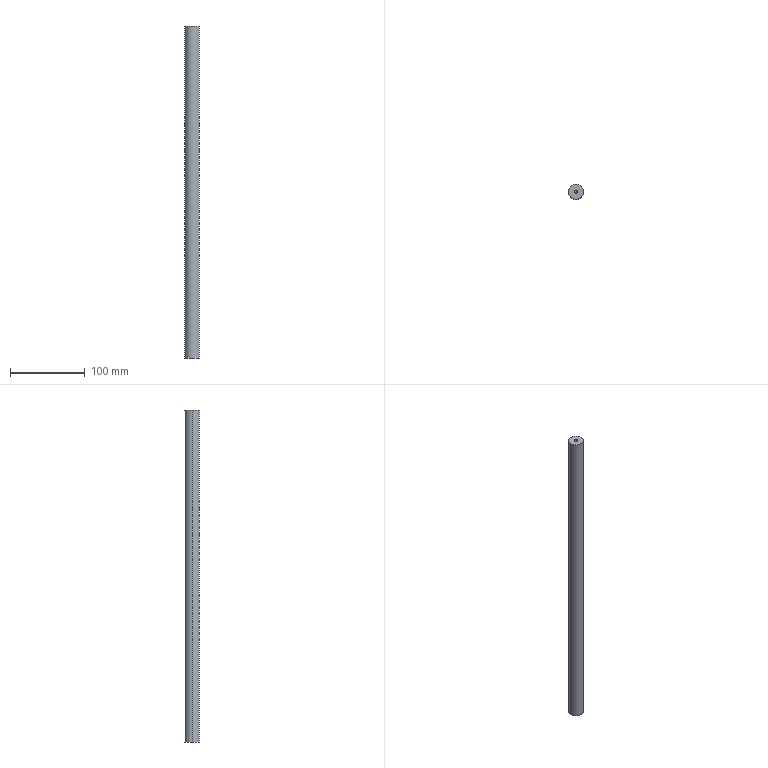Part | SolidWorks | features HoleWzd 2, Extrusion 1 | 1 solid | 12 faces | box 20 x 20 x 445 mm | volume 139374 mm3 | cylinder 6 | cone 4 | plane 2 | commonest cylinder face diameters 4.2 x4 20 x2
STEP:
#1=CARTESIAN_POINT('',(2.1,0.,15.));
#2=VERTEX_POINT('',#1);
#3=CARTESIAN_POINT('',(-2.1,0.,15.));
#4=VERTEX_POINT('',#3);
#5=CARTESIAN_POINT('',(0.,0.,15.));
#6=DIRECTION('',(0.,0.,-1.));
#7=DIRECTION('',(-1.,0.,0.));
#8=AXIS2_PLACEMENT_3D('',#5,#6,#7);
#9=CIRCLE('',#8,2.1);
#10=EDGE_CURVE('',#2,#4,#9,.T.);
#11=ORIENTED_EDGE('',*,*,#10,.F.);
#12=CARTESIAN_POINT('',(2.1,0.,0.));
#13=VERTEX_POINT('',#12);
#14=CARTESIAN_POINT('',(2.1,0.,0.));
#15=DIRECTION('',(0.,0.,-1.));
#16=VECTOR('',#15,1000.);
#17=LINE('',#14,#16);
#18=EDGE_CURVE('',#2,#13,#17,.T.);
#19=ORIENTED_EDGE('',*,*,#18,.T.);
#20=CARTESIAN_POINT('',(-2.1,0.,0.));
#21=VERTEX_POINT('',#20);
#22=CARTESIAN_POINT('',(0.,0.,0.));
#23=DIRECTION('',(0.,0.,-1.));
#24=DIRECTION('',(-1.,0.,0.));
#25=AXIS2_PLACEMENT_3D('',#22,#23,#24);
#26=CIRCLE('',#25,2.1);
#27=EDGE_CURVE('',#13,#21,#26,.T.);
#28=ORIENTED_EDGE('',*,*,#27,.T.);
#29=CARTESIAN_POINT('',(-2.1,0.,0.));
#30=DIRECTION('',(0.,0.,-1.));
#31=VECTOR('',#30,1000.);
#32=LINE('',#29,#31);
#33=EDGE_CURVE('',#4,#21,#32,.T.);
#34=ORIENTED_EDGE('',*,*,#33,.F.);
#35=EDGE_LOOP('',(#11,#19,#28,#34));
#36=FACE_OUTER_BOUND('',#35,.T.);
#37=CARTESIAN_POINT('',(0.,0.,0.));
#38=DIRECTION('',(0.,0.,-1.));
#39=DIRECTION('',(-1.,0.,0.));
#40=AXIS2_PLACEMENT_3D('',#37,#38,#39);
#41=CYLINDRICAL_SURFACE('',#40,2.1);
#42=ADVANCED_FACE('',(#36),#41,.F.);
#43=CARTESIAN_POINT('',(0.,0.,16.262));
#44=VERTEX_POINT('',#43);
#45=CARTESIAN_POINT('',(-2.1,0.,15.));
#46=DIRECTION('',(-0.8572,0.,-0.515));
#47=VECTOR('',#46,1000.);
#48=LINE('',#45,#47);
#49=EDGE_CURVE('',#44,#4,#48,.T.);
#50=ORIENTED_EDGE('',*,*,#49,.F.);
#51=CARTESIAN_POINT('',(2.1,0.,15.));
#52=DIRECTION('',(0.8572,0.,-0.515));
#53=VECTOR('',#52,1000.);
#54=LINE('',#51,#53);
#55=EDGE_CURVE('',#44,#2,#54,.T.);
#56=ORIENTED_EDGE('',*,*,#55,.T.);
#57=ORIENTED_EDGE('',*,*,#10,.T.);
#58=EDGE_LOOP('',(#50,#56,#57));
#59=FACE_OUTER_BOUND('',#58,.T.);
#60=CARTESIAN_POINT('',(0.,0.,15.));
#61=DIRECTION('',(0.,0.,-1.));
#62=DIRECTION('',(-1.,0.,0.));
#63=AXIS2_PLACEMENT_3D('',#60,#61,#62);
#64=CONICAL_SURFACE('',#63,2.1,1.03);
#65=ADVANCED_FACE('',(#59),#64,.F.);
#66=CARTESIAN_POINT('',(-2.1,0.,430.));
#67=VERTEX_POINT('',#66);
#68=CARTESIAN_POINT('',(2.1,0.,430.));
#69=VERTEX_POINT('',#68);
#70=CARTESIAN_POINT('',(0.,0.,430.));
#71=DIRECTION('',(0.,0.,1.));
#72=DIRECTION('',(1.,0.,0.));
#73=AXIS2_PLACEMENT_3D('',#70,#71,#72);
#74=CIRCLE('',#73,2.1);
#75=EDGE_CURVE('',#67,#69,#74,.T.);
#76=ORIENTED_EDGE('',*,*,#75,.F.);
#77=CARTESIAN_POINT('',(-2.1,0.,445.));
#78=VERTEX_POINT('',#77);
#79=CARTESIAN_POINT('',(-2.1,0.,445.));
#80=DIRECTION('',(0.,0.,1.));
#81=VECTOR('',#80,1000.);
#82=LINE('',#79,#81);
#83=EDGE_CURVE('',#67,#78,#82,.T.);
#84=ORIENTED_EDGE('',*,*,#83,.T.);
#85=CARTESIAN_POINT('',(2.1,0.,445.));
#86=VERTEX_POINT('',#85);
#87=CARTESIAN_POINT('',(0.,0.,445.));
#88=DIRECTION('',(0.,0.,1.));
#89=DIRECTION('',(1.,0.,0.));
#90=AXIS2_PLACEMENT_3D('',#87,#88,#89);
#91=CIRCLE('',#90,2.1);
#92=EDGE_CURVE('',#78,#86,#91,.T.);
#93=ORIENTED_EDGE('',*,*,#92,.T.);
#94=CARTESIAN_POINT('',(2.1,0.,445.));
#95=DIRECTION('',(0.,0.,1.));
#96=VECTOR('',#95,1000.);
#97=LINE('',#94,#96);
#98=EDGE_CURVE('',#69,#86,#97,.T.);
#99=ORIENTED_EDGE('',*,*,#98,.F.);
#100=EDGE_LOOP('',(#76,#84,#93,#99));
#101=FACE_OUTER_BOUND('',#100,.T.);
#102=CARTESIAN_POINT('',(0.,0.,445.));
#103=DIRECTION('',(0.,0.,1.));
#104=DIRECTION('',(1.,0.,0.));
#105=AXIS2_PLACEMENT_3D('',#102,#103,#104);
#106=CYLINDRICAL_SURFACE('',#105,2.1);
#107=ADVANCED_FACE('',(#101),#106,.F.);
#108=CARTESIAN_POINT('',(0.,0.,428.738));
#109=VERTEX_POINT('',#108);
#110=CARTESIAN_POINT('',(2.1,0.,430.));
#111=DIRECTION('',(0.8572,0.,0.515));
#112=VECTOR('',#111,1000.);
#113=LINE('',#110,#112);
#114=EDGE_CURVE('',#109,#69,#113,.T.);
#115=ORIENTED_EDGE('',*,*,#114,.F.);
#116=CARTESIAN_POINT('',(-2.1,0.,430.));
#117=DIRECTION('',(-0.8572,0.,0.515));
#118=VECTOR('',#117,1000.);
#119=LINE('',#116,#118);
#120=EDGE_CURVE('',#109,#67,#119,.T.);
#121=ORIENTED_EDGE('',*,*,#120,.T.);
#122=ORIENTED_EDGE('',*,*,#75,.T.);
#123=EDGE_LOOP('',(#115,#121,#122));
#124=FACE_OUTER_BOUND('',#123,.T.);
#125=CARTESIAN_POINT('',(0.,0.,430.));
#126=DIRECTION('',(0.,0.,1.));
#127=DIRECTION('',(1.,0.,0.));
#128=AXIS2_PLACEMENT_3D('',#125,#126,#127);
#129=CONICAL_SURFACE('',#128,2.1,1.03);
#130=ADVANCED_FACE('',(#124),#129,.F.);
#131=CARTESIAN_POINT('',(10.,0.,445.));
#132=VERTEX_POINT('',#131);
#133=CARTESIAN_POINT('',(-10.,0.,445.));
#134=VERTEX_POINT('',#133);
#135=CARTESIAN_POINT('',(0.,0.,445.));
#136=DIRECTION('',(0.,0.,1.));
#137=DIRECTION('',(1.,0.,0.));
#138=AXIS2_PLACEMENT_3D('',#135,#136,#137);
#139=CIRCLE('',#138,10.);
#140=EDGE_CURVE('',#132,#134,#139,.T.);
#141=ORIENTED_EDGE('',*,*,#140,.F.);
#142=CARTESIAN_POINT('',(10.,0.,0.));
#143=VERTEX_POINT('',#142);
#144=CARTESIAN_POINT('',(10.,0.,445.));
#145=DIRECTION('',(0.,0.,-1.));
#146=VECTOR('',#145,1000.);
#147=LINE('',#144,#146);
#148=EDGE_CURVE('',#132,#143,#147,.T.);
#149=ORIENTED_EDGE('',*,*,#148,.T.);
#150=CARTESIAN_POINT('',(-10.,0.,0.));
#151=VERTEX_POINT('',#150);
#152=CARTESIAN_POINT('',(0.,0.,0.));
#153=DIRECTION('',(0.,0.,1.));
#154=DIRECTION('',(1.,0.,0.));
#155=AXIS2_PLACEMENT_3D('',#152,#153,#154);
#156=CIRCLE('',#155,10.);
#157=EDGE_CURVE('',#143,#151,#156,.T.);
#158=ORIENTED_EDGE('',*,*,#157,.T.);
#159=CARTESIAN_POINT('',(-10.,0.,445.));
#160=DIRECTION('',(0.,0.,-1.));
#161=VECTOR('',#160,1000.);
#162=LINE('',#159,#161);
#163=EDGE_CURVE('',#134,#151,#162,.T.);
#164=ORIENTED_EDGE('',*,*,#163,.F.);
#165=EDGE_LOOP('',(#141,#149,#158,#164));
#166=FACE_OUTER_BOUND('',#165,.T.);
#167=CARTESIAN_POINT('',(0.,0.,445.));
#168=DIRECTION('',(0.,0.,-1.));
#169=DIRECTION('',(-1.,0.,0.));
#170=AXIS2_PLACEMENT_3D('',#167,#168,#169);
#171=CYLINDRICAL_SURFACE('',#170,10.);
#172=ADVANCED_FACE('',(#166),#171,.T.);
#173=ORIENTED_EDGE('',*,*,#148,.F.);
#174=CARTESIAN_POINT('',(0.,0.,445.));
#175=DIRECTION('',(0.,0.,1.));
#176=DIRECTION('',(1.,0.,0.));
#177=AXIS2_PLACEMENT_3D('',#174,#175,#176);
#178=CIRCLE('',#177,10.);
#179=EDGE_CURVE('',#134,#132,#178,.T.);
#180=ORIENTED_EDGE('',*,*,#179,.F.);
#181=ORIENTED_EDGE('',*,*,#163,.T.);
#182=CARTESIAN_POINT('',(0.,0.,0.));
#183=DIRECTION('',(0.,0.,1.));
#184=DIRECTION('',(1.,0.,0.));
#185=AXIS2_PLACEMENT_3D('',#182,#183,#184);
#186=CIRCLE('',#185,10.);
#187=EDGE_CURVE('',#151,#143,#186,.T.);
#188=ORIENTED_EDGE('',*,*,#187,.T.);
#189=EDGE_LOOP('',(#173,#180,#181,#188));
#190=FACE_OUTER_BOUND('',#189,.T.);
#191=CARTESIAN_POINT('',(0.,0.,445.));
#192=DIRECTION('',(0.,0.,-1.));
#193=DIRECTION('',(-1.,0.,0.));
#194=AXIS2_PLACEMENT_3D('',#191,#192,#193);
#195=CYLINDRICAL_SURFACE('',#194,10.);
#196=ADVANCED_FACE('',(#190),#195,.T.);
#197=CARTESIAN_POINT('',(0.,0.,445.));
#198=DIRECTION('',(0.,0.,1.));
#199=DIRECTION('',(1.,0.,0.));
#200=AXIS2_PLACEMENT_3D('',#197,#198,#199);
#201=CIRCLE('',#200,2.1);
#202=EDGE_CURVE('',#86,#78,#201,.T.);
#203=ORIENTED_EDGE('',*,*,#202,.F.);
#204=ORIENTED_EDGE('',*,*,#92,.F.);
#205=EDGE_LOOP('',(#203,#204));
#206=FACE_BOUND('',#205,.T.);
#207=ORIENTED_EDGE('',*,*,#179,.T.);
#208=ORIENTED_EDGE('',*,*,#140,.T.);
#209=EDGE_LOOP('',(#207,#208));
#210=FACE_OUTER_BOUND('',#209,.T.);
#211=CARTESIAN_POINT('',(0.,0.,445.));
#212=DIRECTION('',(0.,0.,1.));
#213=DIRECTION('',(1.,0.,0.));
#214=AXIS2_PLACEMENT_3D('',#211,#212,#213);
#215=PLANE('',#214);
#216=ADVANCED_FACE('',(#206,#210),#215,.T.);
#217=CARTESIAN_POINT('',(0.,0.,0.));
#218=DIRECTION('',(0.,0.,-1.));
#219=DIRECTION('',(-1.,0.,0.));
#220=AXIS2_PLACEMENT_3D('',#217,#218,#219);
#221=CIRCLE('',#220,2.1);
#222=EDGE_CURVE('',#21,#13,#221,.T.);
#223=ORIENTED_EDGE('',*,*,#222,.F.);
#224=ORIENTED_EDGE('',*,*,#27,.F.);
#225=EDGE_LOOP('',(#223,#224));
#226=FACE_BOUND('',#225,.T.);
#227=ORIENTED_EDGE('',*,*,#187,.F.);
#228=ORIENTED_EDGE('',*,*,#157,.F.);
#229=EDGE_LOOP('',(#227,#228));
#230=FACE_OUTER_BOUND('',#229,.T.);
#231=CARTESIAN_POINT('',(0.,0.,0.));
#232=DIRECTION('',(0.,0.,1.));
#233=DIRECTION('',(1.,0.,0.));
#234=AXIS2_PLACEMENT_3D('',#231,#232,#233);
#235=PLANE('',#234);
#236=ADVANCED_FACE('',(#226,#230),#235,.F.);
#237=ORIENTED_EDGE('',*,*,#120,.F.);
#238=ORIENTED_EDGE('',*,*,#114,.T.);
#239=CARTESIAN_POINT('',(0.,0.,430.));
#240=DIRECTION('',(0.,0.,1.));
#241=DIRECTION('',(1.,0.,0.));
#242=AXIS2_PLACEMENT_3D('',#239,#240,#241);
#243=CIRCLE('',#242,2.1);
#244=EDGE_CURVE('',#69,#67,#243,.T.);
#245=ORIENTED_EDGE('',*,*,#244,.T.);
#246=EDGE_LOOP('',(#237,#238,#245));
#247=FACE_OUTER_BOUND('',#246,.T.);
#248=CARTESIAN_POINT('',(0.,0.,430.));
#249=DIRECTION('',(0.,0.,1.));
#250=DIRECTION('',(1.,0.,0.));
#251=AXIS2_PLACEMENT_3D('',#248,#249,#250);
#252=CONICAL_SURFACE('',#251,2.1,1.03);
#253=ADVANCED_FACE('',(#247),#252,.F.);
#254=ORIENTED_EDGE('',*,*,#83,.F.);
#255=ORIENTED_EDGE('',*,*,#244,.F.);
#256=ORIENTED_EDGE('',*,*,#98,.T.);
#257=ORIENTED_EDGE('',*,*,#202,.T.);
#258=EDGE_LOOP('',(#254,#255,#256,#257));
#259=FACE_OUTER_BOUND('',#258,.T.);
#260=CARTESIAN_POINT('',(0.,0.,445.));
#261=DIRECTION('',(0.,0.,1.));
#262=DIRECTION('',(1.,0.,0.));
#263=AXIS2_PLACEMENT_3D('',#260,#261,#262);
#264=CYLINDRICAL_SURFACE('',#263,2.1);
#265=ADVANCED_FACE('',(#259),#264,.F.);
#266=ORIENTED_EDGE('',*,*,#55,.F.);
#267=ORIENTED_EDGE('',*,*,#49,.T.);
#268=CARTESIAN_POINT('',(0.,0.,15.));
#269=DIRECTION('',(0.,0.,-1.));
#270=DIRECTION('',(-1.,0.,0.));
#271=AXIS2_PLACEMENT_3D('',#268,#269,#270);
#272=CIRCLE('',#271,2.1);
#273=EDGE_CURVE('',#4,#2,#272,.T.);
#274=ORIENTED_EDGE('',*,*,#273,.T.);
#275=EDGE_LOOP('',(#266,#267,#274));
#276=FACE_OUTER_BOUND('',#275,.T.);
#277=CARTESIAN_POINT('',(0.,0.,15.));
#278=DIRECTION('',(0.,0.,-1.));
#279=DIRECTION('',(-1.,0.,0.));
#280=AXIS2_PLACEMENT_3D('',#277,#278,#279);
#281=CONICAL_SURFACE('',#280,2.1,1.03);
#282=ADVANCED_FACE('',(#276),#281,.F.);
#283=ORIENTED_EDGE('',*,*,#18,.F.);
#284=ORIENTED_EDGE('',*,*,#273,.F.);
#285=ORIENTED_EDGE('',*,*,#33,.T.);
#286=ORIENTED_EDGE('',*,*,#222,.T.);
#287=EDGE_LOOP('',(#283,#284,#285,#286));
#288=FACE_OUTER_BOUND('',#287,.T.);
#289=CARTESIAN_POINT('',(0.,0.,0.));
#290=DIRECTION('',(0.,0.,-1.));
#291=DIRECTION('',(-1.,0.,0.));
#292=AXIS2_PLACEMENT_3D('',#289,#290,#291);
#293=CYLINDRICAL_SURFACE('',#292,2.1);
#294=ADVANCED_FACE('',(#288),#293,.F.);
#295=CLOSED_SHELL('',(#42,#65,#107,#130,#172,#196,#216,#236,#253,#265,#282,#294));
#296=MANIFOLD_SOLID_BREP('',#295);
#297=CARTESIAN_POINT('',(0.,0.,0.));
#298=DIRECTION('',(0.,0.,1.));
#299=DIRECTION('',(1.,0.,0.));
#300=AXIS2_PLACEMENT_3D('',#297,#298,#299);
#301=(LENGTH_UNIT()NAMED_UNIT(*)SI_UNIT(.MILLI.,.METRE.));
#302=UNCERTAINTY_MEASURE_WITH_UNIT(LENGTH_MEASURE(0.00001),#301,'','');
#303=(NAMED_UNIT(*)PLANE_ANGLE_UNIT()SI_UNIT($,.RADIAN.));
#304=(NAMED_UNIT(*)SI_UNIT($,.STERADIAN.)SOLID_ANGLE_UNIT());
#305=(GEOMETRIC_REPRESENTATION_CONTEXT(3)GLOBAL_UNCERTAINTY_ASSIGNED_CONTEXT((#302))GLOBAL_UNIT_ASSIGNED_CONTEXT((#301,#303,#304))REPRESENTATION_CONTEXT('',''));
#306=ADVANCED_BREP_SHAPE_REPRESENTATION('',(#296,#300),#305);